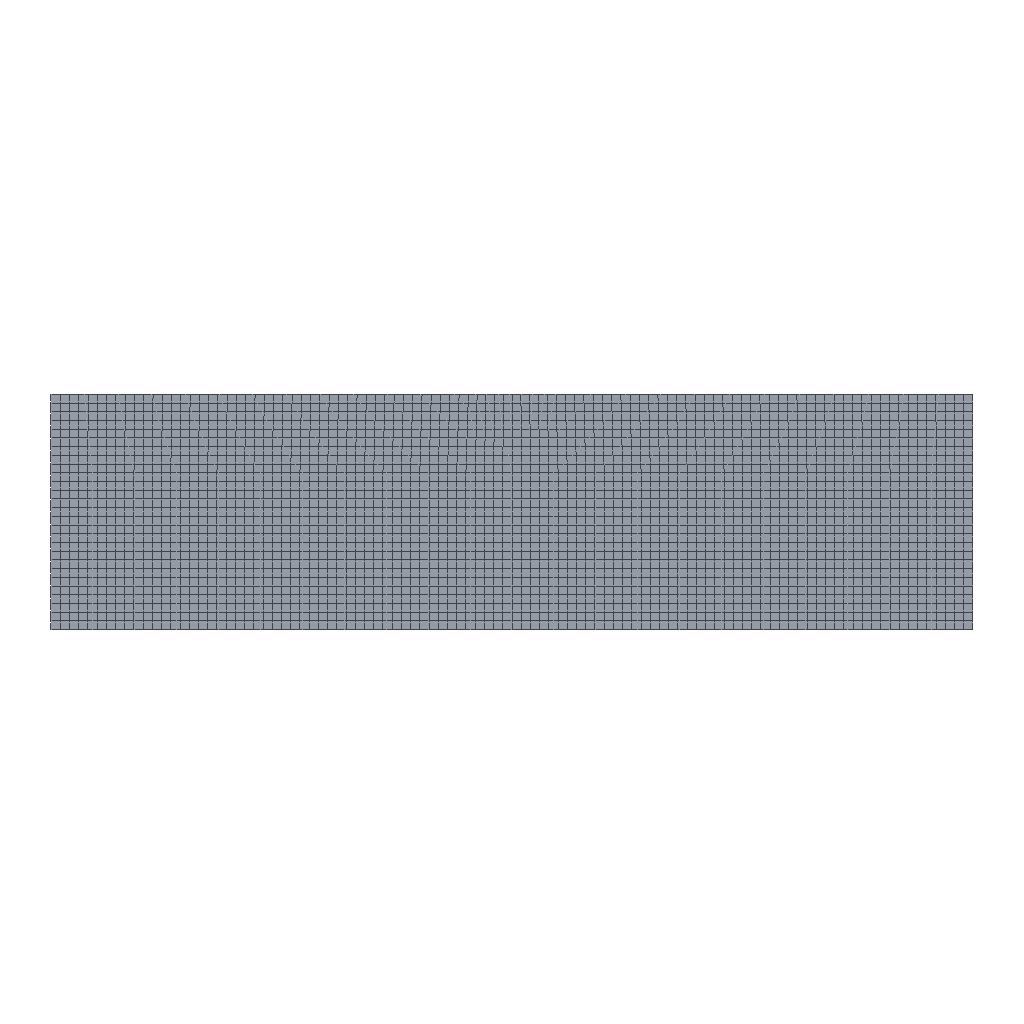Simulation study | abaqus
Set-up summary:
category,name,step,type,value,unit,region
solver,abaqus
solver,version,,,Abaqus/Standard 2020
units,not stated in the deck,,not stated
analysis,deck,,static,static
load_step,Step-1,Step-1,static
load_step,requested,,,1
mesh,nodes,,,2874
mesh,elements,,,2744
element_type,R2D2,,rigid,44
element_type,CPS4R,,plane,2700
load,load commands in deck,,count,1
bc,support commands in deck,,count,4
material,HEISHAYAN,,in results
material,HONGSHAYAN,,in results
material,QINGSHAYAN,,in results
check,setup vs results,,match,"per instance, exact: element labels, types and connectivity; labels of the nodes the elements use; coordinates of those nodes at SINGLE_PRECISION in 3 of 3 instance(s)"
Abaqus input file, long lists of numbers shortened:
*Heading
** Job name: Job-1 Model name: Model-1
** Generated by: Abaqus/CAE 2020
*Preprint, echo=NO, model=NO, history=NO, contact=NO
**
** PARTS
**
*Part, name=Part-1
*Node
      1,           0.,         -17.
      2,         200.,         -17.
** (2826 more lines like these left out)
*Element, type=CPS4R
  1,    1,   11,  453,  222
  2,   11,   12,  454,  453
** (2698 more lines like these left out)
*Nset, nset=Set-3
    1,    2,    3,    4,    5,    6,   11,   12,   13,   14,   15,   16,   17,   18,   19,   20
   21,   22,   23,   24,   25,   26,   27,   28,   29,   30,   31,   32,   33,   34,   35,   36
** (62 more lines like these left out)
*Elset, elset=Set-3, generate
   1,  900,    1
*Nset, nset=Set-4
    1,    2,    7,    8,   11,   12,   13,   14,   15,   16,   17,   18,   19,   20,   21,   22
   23,   24,   25,   26,   27,   28,   29,   30,   31,   32,   33,   34,   35,   36,   37,   38
** (62 more lines like these left out)
*Elset, elset=Set-4, generate
 1801,  2700,     1
*Nset, nset=Set-5
    7,    8,    9,   10,  223,  224,  225,  226,  227,  228,  229,  230,  231,  232,  233,  234
  235,  236,  237,  238,  239,  240,  241,  242,  243,  244,  245,  246,  247,  248,  249,  250
** (62 more lines like these left out)
*Elset, elset=Set-5, generate
  901,  1800,     1
** Section: heishayan
*Solid Section, elset=Set-3, material=heishayan
,
** Section: qingshayan
*Solid Section, elset=Set-5, material=qingshayan
,
** Section: honhshayan
*Solid Section, elset=Set-4, material=hongshayan
,
*End Part
**
*Part, name=crack
*End Part
**
*Part, name=rigid
*Node
      1,          1.5,          -2.
      2,   2.003,  -1.496
** (20 more lines like these left out)
*Element, type=R2D2
 1,  1,  2
 2,  2,  3
** (20 more lines like these left out)
*Node
     23,           0., 1.5308085e-16,           0.
*Nset, nset=rigid-RefPt_, internal
23,
*Elset, elset=rigid, generate
  1,  22,   1
*End Part
**
**
** ASSEMBLY
**
*Assembly, name=Assembly
**
*Instance, name=Part-1-1, part=Part-1
*End Instance
**
*Instance, name=rigid-1, part=rigid
         10.,        -53.5,           0.
*End Instance
**
*Instance, name=rigid-1-lin-2-1, part=rigid
        190.,        -53.5,           0.
*End Instance
**
*Instance, name=crack-1, part=crack
       100.1,         -46.,           0.
*End Instance
**
*Node
      1,   100.045,           0.,           0.
*Nset, nset=Set-1, instance=rigid-1
 23,
*Nset, nset=Set-1, instance=rigid-1-lin-2-1
 23,
*Nset, nset=Set-3
 1,
*Nset, nset=m_Set-2
 1,
*Nset, nset=_PickedSet18, internal, instance=Part-1-1, generate
    1,  2828,     1
*Elset, elset=_PickedSet18, internal, instance=Part-1-1, generate
    1,  2700,     1
*Elset, elset=_m_Surf-2_SNEG, internal, instance=rigid-1, generate
  1,  22,   1
*Elset, elset=_m_Surf-2_SNEG, internal, instance=rigid-1-lin-2-1, generate
  1,  22,   1
*Surface, type=ELEMENT, name=m_Surf-2
_m_Surf-2_SNEG, SNEG
*Elset, elset=_s_Surf-1_S3, internal, instance=Part-1-1, generate
 846,  855,    1
*Surface, type=ELEMENT, name=s_Surf-1
_s_Surf-1_S3, S3
*Elset, elset=_s_Surf-2_S3, internal, instance=Part-1-1, generate
 1701,  1800,     1
*Surface, type=ELEMENT, name=s_Surf-2
_s_Surf-2_S3, S3
*Rigid Body, ref node=rigid-1.rigid-RefPt_, elset=rigid-1.rigid
*Rigid Body, ref node=rigid-1-lin-2-1.rigid-RefPt_, elset=rigid-1-lin-2-1.rigid
** Constraint: Constraint-1
*Coupling, constraint name=Constraint-1, ref node=m_Set-2, surface=s_Surf-1
*Kinematic
*Enrichment, name=Crack-1, type=PROPAGATION CRACK, elset=_PickedSet18
*End Assembly
*Amplitude, name=Amp-1
             0.,              0.,              1.,              1.
**
** MATERIALS
**
*Material, name=heishayan
*Damage Initiation, criterion=QUADE
 0.001, 0.001, 0.001
*Damage Evolution, type=DISPLACEMENT
 1e-06,
*Damage Stabilization
0.001
*Density
 2.475e-09,
*Elastic
33800., 0.21
*Material, name=hongshayan
*Damage Initiation, criterion=QUADE
 0.001, 0.001, 0.001
*Damage Evolution, type=DISPLACEMENT
 0.0001,
*Damage Stabilization
0.001
*Density
 2.317e-09,
*Elastic
24500., 0.19
*Material, name=qingshayan
*Damage Initiation, criterion=QUADE
 5e-05, 5e-05, 5e-05
*Damage Evolution, type=DISPLACEMENT
 1e-06,
*Damage Stabilization
0.001
*Density
 2.37e-09,
*Elastic
12500., 0.26
**
** INTERACTION PROPERTIES
**
*Surface Interaction, name=IntProp-1
1.,
*Friction, slip tolerance=0.005
 0.3,
*Surface Behavior, pressure-overclosure=HARD
*Initial Conditions, type=ENRICHMENT
Part-1-1.155, 1,Crack-1, 1.9, 0.6667
Part-1-1.155, 2,Crack-1, -0.1, 0.6667
Part-1-1.155, 3,Crack-1, -0.1, -1.222
Part-1-1.155, 4,Crack-1, 1.9, -1.222
Part-1-1.165, 1,Crack-1, 1.9
Part-1-1.165, 2,Crack-1, -0.1
Part-1-1.165, 3,Crack-1, -0.1
Part-1-1.165, 4,Crack-1, 1.9
Part-1-1.175, 1,Crack-1, 1.9
Part-1-1.175, 2,Crack-1, -0.1
Part-1-1.175, 3,Crack-1, -0.1
Part-1-1.175, 4,Crack-1, 1.9
**
** INTERACTIONS
**
** Interaction: Int-1
*Contact Pair, interaction=IntProp-1, type=SURFACE TO SURFACE
s_Surf-2, m_Surf-2
** ----------------------------------------------------------------
**
** STEP: Step-1
**
*Step, name=Step-1, nlgeom=YES, inc=1000
*Static, stabilize=0.0002, allsdtol=0.05, continue=NO
0.01, 1., 1e-05, 1.
**
** BOUNDARY CONDITIONS
**
** Name: BC-1 Type: 对称/反对称/完全固定
*Boundary
Set-1, ENCASTRE
** Name: BC-2 Type: 位移/转角
*Boundary, amplitude=Amp-1
Set-3, 1, 1
Set-3, 2, 2, -5.
Set-3, 6, 6
**
** OUTPUT REQUESTS
**
*Restart, write, frequency=0
**
** FIELD OUTPUT: F-Output-1
**
*Output, field
*Node Output
CF, PHILSM, PSILSM, RF, U, V
*Element Output, directions=YES
E, ENRRTXFEM, LE, LOADSXFEM, MISES, MISESMAX, PE, PEEQ, PEMAG, S, SDEG, SSAVG, STATUS, STATUSXFEM
*Contact Output
CDISP, CSTRESS
**
** HISTORY OUTPUT: H-Output-1
**
*Output, history, variable=PRESELECT
*End Step
Results summary:
result,step,,partial,increments=157 time=0.04832/1.0
result,analysis,,,static
result,last_loadstep,,,1
result,primary field,,,U
result,reaction total,,FX,-0.0,model units
result,reaction total,,FY,-8e-06,model units
result,reaction total,,FZ,0.0,model units